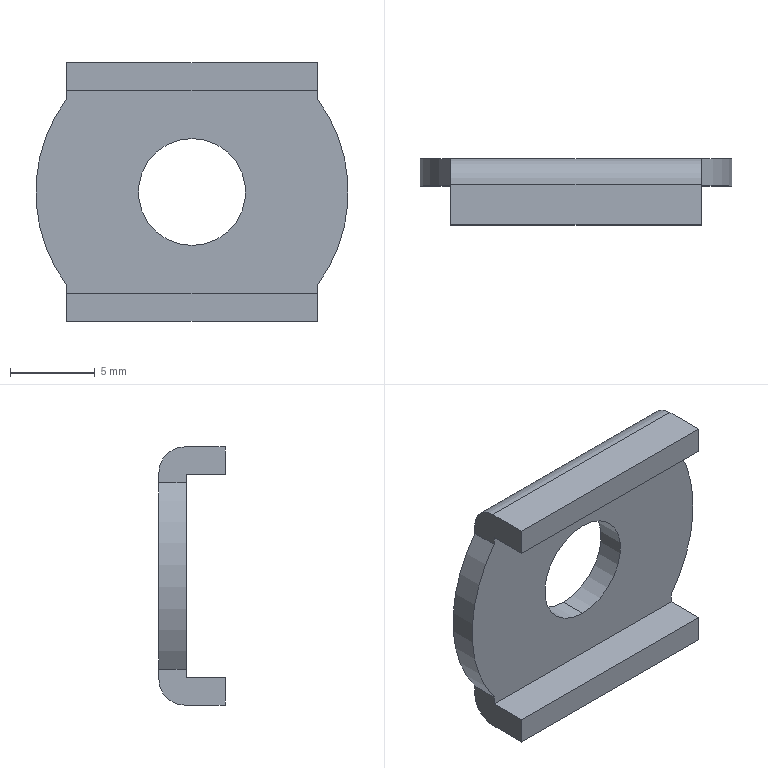Part | STEP file | 11-CLMP_MC01-S311 | 1 solid | 18 faces | box 18.4 x 3.9 x 15.2 mm | volume 446.915 mm3 | plane 12 | cylinder 6 | commonest cylinder face diameters 3 x2 6.3 x2 18.4 x2
STEP:
#1=CARTESIAN_POINT('',(0.,-1.6,-3.15));
#2=VERTEX_POINT('',#1);
#3=CARTESIAN_POINT('',(0.,-1.6,3.15));
#4=VERTEX_POINT('',#3);
#5=CARTESIAN_POINT('',(0.,-1.6,0.));
#6=DIRECTION('',(0.,1.,0.));
#7=DIRECTION('',(0.,0.,1.));
#8=AXIS2_PLACEMENT_3D('',#5,#6,#7);
#9=CIRCLE('',#8,3.15);
#10=EDGE_CURVE('',#2,#4,#9,.T.);
#11=ORIENTED_EDGE('',*,*,#10,.F.);
#12=CARTESIAN_POINT('',(0.,0.,-3.15));
#13=VERTEX_POINT('',#12);
#14=CARTESIAN_POINT('',(0.,0.,-3.15));
#15=DIRECTION('',(0.,1.,0.));
#16=VECTOR('',#15,1000.);
#17=LINE('',#14,#16);
#18=EDGE_CURVE('',#2,#13,#17,.T.);
#19=ORIENTED_EDGE('',*,*,#18,.T.);
#20=CARTESIAN_POINT('',(0.,0.,3.15));
#21=VERTEX_POINT('',#20);
#22=CARTESIAN_POINT('',(0.,0.,0.));
#23=DIRECTION('',(0.,1.,0.));
#24=DIRECTION('',(0.,0.,1.));
#25=AXIS2_PLACEMENT_3D('',#22,#23,#24);
#26=CIRCLE('',#25,3.15);
#27=EDGE_CURVE('',#13,#21,#26,.T.);
#28=ORIENTED_EDGE('',*,*,#27,.T.);
#29=CARTESIAN_POINT('',(0.,0.,3.15));
#30=DIRECTION('',(0.,1.,0.));
#31=VECTOR('',#30,1000.);
#32=LINE('',#29,#31);
#33=EDGE_CURVE('',#4,#21,#32,.T.);
#34=ORIENTED_EDGE('',*,*,#33,.F.);
#35=EDGE_LOOP('',(#11,#19,#28,#34));
#36=FACE_OUTER_BOUND('',#35,.T.);
#37=CARTESIAN_POINT('',(0.,0.,0.));
#38=DIRECTION('',(0.,1.,0.));
#39=DIRECTION('',(0.,0.,1.));
#40=AXIS2_PLACEMENT_3D('',#37,#38,#39);
#41=CYLINDRICAL_SURFACE('',#40,3.15);
#42=ADVANCED_FACE('',(#36),#41,.F.);
#43=CARTESIAN_POINT('',(-7.375,-1.6,-5.5));
#44=VERTEX_POINT('',#43);
#45=CARTESIAN_POINT('',(-7.375,0.,-5.5));
#46=VERTEX_POINT('',#45);
#47=CARTESIAN_POINT('',(-7.375,-3.9,-5.5));
#48=DIRECTION('',(0.,1.,0.));
#49=VECTOR('',#48,1000.);
#50=LINE('',#47,#49);
#51=EDGE_CURVE('',#44,#46,#50,.T.);
#52=ORIENTED_EDGE('',*,*,#51,.F.);
#53=CARTESIAN_POINT('',(-7.375,-1.6,5.5));
#54=VERTEX_POINT('',#53);
#55=CARTESIAN_POINT('',(0.,-1.6,0.));
#56=DIRECTION('',(0.,1.,0.));
#57=DIRECTION('',(0.,0.,1.));
#58=AXIS2_PLACEMENT_3D('',#55,#56,#57);
#59=CIRCLE('',#58,9.2);
#60=EDGE_CURVE('',#44,#54,#59,.T.);
#61=ORIENTED_EDGE('',*,*,#60,.T.);
#62=CARTESIAN_POINT('',(-7.375,0.,5.5));
#63=VERTEX_POINT('',#62);
#64=CARTESIAN_POINT('',(-7.375,-3.9,5.5));
#65=DIRECTION('',(0.,1.,0.));
#66=VECTOR('',#65,1000.);
#67=LINE('',#64,#66);
#68=EDGE_CURVE('',#54,#63,#67,.T.);
#69=ORIENTED_EDGE('',*,*,#68,.T.);
#70=CARTESIAN_POINT('',(0.,0.,0.));
#71=DIRECTION('',(0.,1.,0.));
#72=DIRECTION('',(0.,0.,1.));
#73=AXIS2_PLACEMENT_3D('',#70,#71,#72);
#74=CIRCLE('',#73,9.2);
#75=EDGE_CURVE('',#46,#63,#74,.T.);
#76=ORIENTED_EDGE('',*,*,#75,.F.);
#77=EDGE_LOOP('',(#52,#61,#69,#76));
#78=FACE_OUTER_BOUND('',#77,.T.);
#79=CARTESIAN_POINT('',(0.,-3.9,0.));
#80=DIRECTION('',(0.,1.,0.));
#81=DIRECTION('',(0.,0.,1.));
#82=AXIS2_PLACEMENT_3D('',#79,#80,#81);
#83=CYLINDRICAL_SURFACE('',#82,9.2);
#84=ADVANCED_FACE('',(#78),#83,.T.);
#85=CARTESIAN_POINT('',(-7.375,-3.9,-6.));
#86=VERTEX_POINT('',#85);
#87=CARTESIAN_POINT('',(-7.375,-1.6,-6.));
#88=VERTEX_POINT('',#87);
#89=CARTESIAN_POINT('',(-7.375,-3.9,-6.));
#90=DIRECTION('',(0.,1.,0.));
#91=VECTOR('',#90,1000.);
#92=LINE('',#89,#91);
#93=EDGE_CURVE('',#86,#88,#92,.T.);
#94=ORIENTED_EDGE('',*,*,#93,.T.);
#95=CARTESIAN_POINT('',(-7.375,-1.6,0.));
#96=DIRECTION('',(0.,0.,1.));
#97=VECTOR('',#96,1000.);
#98=LINE('',#95,#97);
#99=EDGE_CURVE('',#88,#44,#98,.T.);
#100=ORIENTED_EDGE('',*,*,#99,.T.);
#101=ORIENTED_EDGE('',*,*,#51,.T.);
#102=CARTESIAN_POINT('',(-7.375,0.,-6.1));
#103=VERTEX_POINT('',#102);
#104=CARTESIAN_POINT('',(-7.375,0.,-5.5));
#105=DIRECTION('',(0.,0.,1.));
#106=VECTOR('',#105,1000.);
#107=LINE('',#104,#106);
#108=EDGE_CURVE('',#103,#46,#107,.T.);
#109=ORIENTED_EDGE('',*,*,#108,.F.);
#110=CARTESIAN_POINT('',(-7.375,-1.5,-7.6));
#111=VERTEX_POINT('',#110);
#112=CARTESIAN_POINT('',(-7.375,-1.5,-6.1));
#113=DIRECTION('',(-1.,0.,0.));
#114=DIRECTION('',(0.,0.,1.));
#115=AXIS2_PLACEMENT_3D('',#112,#113,#114);
#116=CIRCLE('',#115,1.5);
#117=EDGE_CURVE('',#103,#111,#116,.T.);
#118=ORIENTED_EDGE('',*,*,#117,.T.);
#119=CARTESIAN_POINT('',(-7.375,-3.9,-7.6));
#120=VERTEX_POINT('',#119);
#121=CARTESIAN_POINT('',(-7.375,-3.9,-7.6));
#122=DIRECTION('',(0.,1.,0.));
#123=VECTOR('',#122,1000.);
#124=LINE('',#121,#123);
#125=EDGE_CURVE('',#120,#111,#124,.T.);
#126=ORIENTED_EDGE('',*,*,#125,.F.);
#127=CARTESIAN_POINT('',(-7.375,-3.9,-5.5));
#128=DIRECTION('',(0.,0.,1.));
#129=VECTOR('',#128,1000.);
#130=LINE('',#127,#129);
#131=EDGE_CURVE('',#120,#86,#130,.T.);
#132=ORIENTED_EDGE('',*,*,#131,.T.);
#133=EDGE_LOOP('',(#94,#100,#101,#109,#118,#126,#132));
#134=FACE_OUTER_BOUND('',#133,.T.);
#135=CARTESIAN_POINT('',(-7.375,-3.9,-5.5));
#136=DIRECTION('',(-1.,0.,0.));
#137=DIRECTION('',(0.,0.,1.));
#138=AXIS2_PLACEMENT_3D('',#135,#136,#137);
#139=PLANE('',#138);
#140=ADVANCED_FACE('',(#134),#139,.T.);
#141=CARTESIAN_POINT('',(7.375,-1.6,5.5));
#142=VERTEX_POINT('',#141);
#143=CARTESIAN_POINT('',(7.375,0.,5.5));
#144=VERTEX_POINT('',#143);
#145=CARTESIAN_POINT('',(7.375,-3.9,5.5));
#146=DIRECTION('',(0.,1.,0.));
#147=VECTOR('',#146,1000.);
#148=LINE('',#145,#147);
#149=EDGE_CURVE('',#142,#144,#148,.T.);
#150=ORIENTED_EDGE('',*,*,#149,.F.);
#151=CARTESIAN_POINT('',(7.375,-1.6,-5.5));
#152=VERTEX_POINT('',#151);
#153=CARTESIAN_POINT('',(0.,-1.6,0.));
#154=DIRECTION('',(0.,1.,0.));
#155=DIRECTION('',(0.,0.,1.));
#156=AXIS2_PLACEMENT_3D('',#153,#154,#155);
#157=CIRCLE('',#156,9.2);
#158=EDGE_CURVE('',#142,#152,#157,.T.);
#159=ORIENTED_EDGE('',*,*,#158,.T.);
#160=CARTESIAN_POINT('',(7.375,0.,-5.5));
#161=VERTEX_POINT('',#160);
#162=CARTESIAN_POINT('',(7.375,-3.9,-5.5));
#163=DIRECTION('',(0.,1.,0.));
#164=VECTOR('',#163,1000.);
#165=LINE('',#162,#164);
#166=EDGE_CURVE('',#152,#161,#165,.T.);
#167=ORIENTED_EDGE('',*,*,#166,.T.);
#168=CARTESIAN_POINT('',(0.,0.,0.));
#169=DIRECTION('',(0.,1.,0.));
#170=DIRECTION('',(0.,0.,1.));
#171=AXIS2_PLACEMENT_3D('',#168,#169,#170);
#172=CIRCLE('',#171,9.2);
#173=EDGE_CURVE('',#144,#161,#172,.T.);
#174=ORIENTED_EDGE('',*,*,#173,.F.);
#175=EDGE_LOOP('',(#150,#159,#167,#174));
#176=FACE_OUTER_BOUND('',#175,.T.);
#177=CARTESIAN_POINT('',(0.,-3.9,0.));
#178=DIRECTION('',(0.,1.,0.));
#179=DIRECTION('',(0.,0.,1.));
#180=AXIS2_PLACEMENT_3D('',#177,#178,#179);
#181=CYLINDRICAL_SURFACE('',#180,9.2);
#182=ADVANCED_FACE('',(#176),#181,.T.);
#183=CARTESIAN_POINT('',(7.375,-3.9,6.));
#184=VERTEX_POINT('',#183);
#185=CARTESIAN_POINT('',(7.375,-1.6,6.));
#186=VERTEX_POINT('',#185);
#187=CARTESIAN_POINT('',(7.375,-3.9,6.));
#188=DIRECTION('',(0.,1.,0.));
#189=VECTOR('',#188,1000.);
#190=LINE('',#187,#189);
#191=EDGE_CURVE('',#184,#186,#190,.T.);
#192=ORIENTED_EDGE('',*,*,#191,.T.);
#193=CARTESIAN_POINT('',(7.375,-1.6,0.));
#194=DIRECTION('',(0.,0.,-1.));
#195=VECTOR('',#194,1000.);
#196=LINE('',#193,#195);
#197=EDGE_CURVE('',#186,#142,#196,.T.);
#198=ORIENTED_EDGE('',*,*,#197,.T.);
#199=ORIENTED_EDGE('',*,*,#149,.T.);
#200=CARTESIAN_POINT('',(7.375,0.,6.1));
#201=VERTEX_POINT('',#200);
#202=CARTESIAN_POINT('',(7.375,0.,7.6));
#203=DIRECTION('',(0.,0.,-1.));
#204=VECTOR('',#203,1000.);
#205=LINE('',#202,#204);
#206=EDGE_CURVE('',#201,#144,#205,.T.);
#207=ORIENTED_EDGE('',*,*,#206,.F.);
#208=CARTESIAN_POINT('',(7.375,-1.5,7.6));
#209=VERTEX_POINT('',#208);
#210=CARTESIAN_POINT('',(7.375,-1.5,6.1));
#211=DIRECTION('',(1.,0.,0.));
#212=DIRECTION('',(0.,0.,-1.));
#213=AXIS2_PLACEMENT_3D('',#210,#211,#212);
#214=CIRCLE('',#213,1.5);
#215=EDGE_CURVE('',#201,#209,#214,.T.);
#216=ORIENTED_EDGE('',*,*,#215,.T.);
#217=CARTESIAN_POINT('',(7.375,-3.9,7.6));
#218=VERTEX_POINT('',#217);
#219=CARTESIAN_POINT('',(7.375,-3.9,7.6));
#220=DIRECTION('',(0.,1.,0.));
#221=VECTOR('',#220,1000.);
#222=LINE('',#219,#221);
#223=EDGE_CURVE('',#218,#209,#222,.T.);
#224=ORIENTED_EDGE('',*,*,#223,.F.);
#225=CARTESIAN_POINT('',(7.375,-3.9,7.6));
#226=DIRECTION('',(0.,0.,-1.));
#227=VECTOR('',#226,1000.);
#228=LINE('',#225,#227);
#229=EDGE_CURVE('',#218,#184,#228,.T.);
#230=ORIENTED_EDGE('',*,*,#229,.T.);
#231=EDGE_LOOP('',(#192,#198,#199,#207,#216,#224,#230));
#232=FACE_OUTER_BOUND('',#231,.T.);
#233=CARTESIAN_POINT('',(7.375,-3.9,7.6));
#234=DIRECTION('',(1.,0.,0.));
#235=DIRECTION('',(0.,0.,-1.));
#236=AXIS2_PLACEMENT_3D('',#233,#234,#235);
#237=PLANE('',#236);
#238=ADVANCED_FACE('',(#232),#237,.T.);
#239=CARTESIAN_POINT('',(7.375,-3.9,-6.));
#240=VERTEX_POINT('',#239);
#241=CARTESIAN_POINT('',(7.375,-3.9,-7.6));
#242=VERTEX_POINT('',#241);
#243=CARTESIAN_POINT('',(7.375,-3.9,-5.5));
#244=DIRECTION('',(0.,0.,-1.));
#245=VECTOR('',#244,1000.);
#246=LINE('',#243,#245);
#247=EDGE_CURVE('',#240,#242,#246,.T.);
#248=ORIENTED_EDGE('',*,*,#247,.F.);
#249=CARTESIAN_POINT('',(0.,-3.9,-6.));
#250=DIRECTION('',(-1.,0.,0.));
#251=VECTOR('',#250,1000.);
#252=LINE('',#249,#251);
#253=EDGE_CURVE('',#240,#86,#252,.T.);
#254=ORIENTED_EDGE('',*,*,#253,.T.);
#255=ORIENTED_EDGE('',*,*,#131,.F.);
#256=CARTESIAN_POINT('',(-7.375,-3.9,-7.6));
#257=DIRECTION('',(-1.,0.,0.));
#258=VECTOR('',#257,1000.);
#259=LINE('',#256,#258);
#260=EDGE_CURVE('',#242,#120,#259,.T.);
#261=ORIENTED_EDGE('',*,*,#260,.F.);
#262=EDGE_LOOP('',(#248,#254,#255,#261));
#263=FACE_OUTER_BOUND('',#262,.T.);
#264=CARTESIAN_POINT('',(0.,-3.9,0.));
#265=DIRECTION('',(0.,1.,0.));
#266=DIRECTION('',(0.,0.,1.));
#267=AXIS2_PLACEMENT_3D('',#264,#265,#266);
#268=PLANE('',#267);
#269=ADVANCED_FACE('',(#263),#268,.F.);
#270=ORIENTED_EDGE('',*,*,#125,.T.);
#271=CARTESIAN_POINT('',(7.375,-1.5,-7.6));
#272=VERTEX_POINT('',#271);
#273=CARTESIAN_POINT('',(-7.375,-1.5,-7.6));
#274=DIRECTION('',(1.,0.,0.));
#275=VECTOR('',#274,1000.);
#276=LINE('',#273,#275);
#277=EDGE_CURVE('',#111,#272,#276,.T.);
#278=ORIENTED_EDGE('',*,*,#277,.T.);
#279=CARTESIAN_POINT('',(7.375,-3.9,-7.6));
#280=DIRECTION('',(0.,1.,0.));
#281=VECTOR('',#280,1000.);
#282=LINE('',#279,#281);
#283=EDGE_CURVE('',#242,#272,#282,.T.);
#284=ORIENTED_EDGE('',*,*,#283,.F.);
#285=ORIENTED_EDGE('',*,*,#260,.T.);
#286=EDGE_LOOP('',(#270,#278,#284,#285));
#287=FACE_OUTER_BOUND('',#286,.T.);
#288=CARTESIAN_POINT('',(-7.375,-3.9,-7.6));
#289=DIRECTION('',(0.,0.,-1.));
#290=DIRECTION('',(-1.,0.,0.));
#291=AXIS2_PLACEMENT_3D('',#288,#289,#290);
#292=PLANE('',#291);
#293=ADVANCED_FACE('',(#287),#292,.T.);
#294=CARTESIAN_POINT('',(7.375,-1.6,-6.));
#295=VERTEX_POINT('',#294);
#296=CARTESIAN_POINT('',(7.375,-3.9,-6.));
#297=DIRECTION('',(0.,1.,0.));
#298=VECTOR('',#297,1000.);
#299=LINE('',#296,#298);
#300=EDGE_CURVE('',#240,#295,#299,.T.);
#301=ORIENTED_EDGE('',*,*,#300,.F.);
#302=ORIENTED_EDGE('',*,*,#247,.T.);
#303=ORIENTED_EDGE('',*,*,#283,.T.);
#304=CARTESIAN_POINT('',(7.375,0.,-6.1));
#305=VERTEX_POINT('',#304);
#306=CARTESIAN_POINT('',(7.375,-1.5,-6.1));
#307=DIRECTION('',(1.,0.,0.));
#308=DIRECTION('',(0.,0.,-1.));
#309=AXIS2_PLACEMENT_3D('',#306,#307,#308);
#310=CIRCLE('',#309,1.5);
#311=EDGE_CURVE('',#272,#305,#310,.T.);
#312=ORIENTED_EDGE('',*,*,#311,.T.);
#313=CARTESIAN_POINT('',(7.375,0.,-5.5));
#314=DIRECTION('',(0.,0.,-1.));
#315=VECTOR('',#314,1000.);
#316=LINE('',#313,#315);
#317=EDGE_CURVE('',#161,#305,#316,.T.);
#318=ORIENTED_EDGE('',*,*,#317,.F.);
#319=ORIENTED_EDGE('',*,*,#166,.F.);
#320=CARTESIAN_POINT('',(7.375,-1.6,0.));
#321=DIRECTION('',(0.,0.,-1.));
#322=VECTOR('',#321,1000.);
#323=LINE('',#320,#322);
#324=EDGE_CURVE('',#152,#295,#323,.T.);
#325=ORIENTED_EDGE('',*,*,#324,.T.);
#326=EDGE_LOOP('',(#301,#302,#303,#312,#318,#319,#325));
#327=FACE_OUTER_BOUND('',#326,.T.);
#328=CARTESIAN_POINT('',(7.375,-3.9,-5.5));
#329=DIRECTION('',(1.,0.,0.));
#330=DIRECTION('',(0.,0.,-1.));
#331=AXIS2_PLACEMENT_3D('',#328,#329,#330);
#332=PLANE('',#331);
#333=ADVANCED_FACE('',(#327),#332,.T.);
#334=ORIENTED_EDGE('',*,*,#223,.T.);
#335=CARTESIAN_POINT('',(-7.375,-1.5,7.6));
#336=VERTEX_POINT('',#335);
#337=CARTESIAN_POINT('',(-7.375,-1.5,7.6));
#338=DIRECTION('',(-1.,0.,0.));
#339=VECTOR('',#338,1000.);
#340=LINE('',#337,#339);
#341=EDGE_CURVE('',#209,#336,#340,.T.);
#342=ORIENTED_EDGE('',*,*,#341,.T.);
#343=CARTESIAN_POINT('',(-7.375,-3.9,7.6));
#344=VERTEX_POINT('',#343);
#345=CARTESIAN_POINT('',(-7.375,-3.9,7.6));
#346=DIRECTION('',(0.,1.,0.));
#347=VECTOR('',#346,1000.);
#348=LINE('',#345,#347);
#349=EDGE_CURVE('',#344,#336,#348,.T.);
#350=ORIENTED_EDGE('',*,*,#349,.F.);
#351=CARTESIAN_POINT('',(-7.375,-3.9,7.6));
#352=DIRECTION('',(1.,0.,0.));
#353=VECTOR('',#352,1000.);
#354=LINE('',#351,#353);
#355=EDGE_CURVE('',#344,#218,#354,.T.);
#356=ORIENTED_EDGE('',*,*,#355,.T.);
#357=EDGE_LOOP('',(#334,#342,#350,#356));
#358=FACE_OUTER_BOUND('',#357,.T.);
#359=CARTESIAN_POINT('',(-7.375,-3.9,7.6));
#360=DIRECTION('',(0.,0.,1.));
#361=DIRECTION('',(1.,0.,0.));
#362=AXIS2_PLACEMENT_3D('',#359,#360,#361);
#363=PLANE('',#362);
#364=ADVANCED_FACE('',(#358),#363,.T.);
#365=CARTESIAN_POINT('',(-7.375,-3.9,6.));
#366=VERTEX_POINT('',#365);
#367=CARTESIAN_POINT('',(-7.375,-1.6,6.));
#368=VERTEX_POINT('',#367);
#369=CARTESIAN_POINT('',(-7.375,-3.9,6.));
#370=DIRECTION('',(0.,1.,0.));
#371=VECTOR('',#370,1000.);
#372=LINE('',#369,#371);
#373=EDGE_CURVE('',#366,#368,#372,.T.);
#374=ORIENTED_EDGE('',*,*,#373,.F.);
#375=CARTESIAN_POINT('',(-7.375,-3.9,7.6));
#376=DIRECTION('',(0.,0.,1.));
#377=VECTOR('',#376,1000.);
#378=LINE('',#375,#377);
#379=EDGE_CURVE('',#366,#344,#378,.T.);
#380=ORIENTED_EDGE('',*,*,#379,.T.);
#381=ORIENTED_EDGE('',*,*,#349,.T.);
#382=CARTESIAN_POINT('',(-7.375,0.,6.1));
#383=VERTEX_POINT('',#382);
#384=CARTESIAN_POINT('',(-7.375,-1.5,6.1));
#385=DIRECTION('',(-1.,0.,0.));
#386=DIRECTION('',(0.,0.,1.));
#387=AXIS2_PLACEMENT_3D('',#384,#385,#386);
#388=CIRCLE('',#387,1.5);
#389=EDGE_CURVE('',#336,#383,#388,.T.);
#390=ORIENTED_EDGE('',*,*,#389,.T.);
#391=CARTESIAN_POINT('',(-7.375,0.,7.6));
#392=DIRECTION('',(0.,0.,1.));
#393=VECTOR('',#392,1000.);
#394=LINE('',#391,#393);
#395=EDGE_CURVE('',#63,#383,#394,.T.);
#396=ORIENTED_EDGE('',*,*,#395,.F.);
#397=ORIENTED_EDGE('',*,*,#68,.F.);
#398=CARTESIAN_POINT('',(-7.375,-1.6,0.));
#399=DIRECTION('',(0.,0.,1.));
#400=VECTOR('',#399,1000.);
#401=LINE('',#398,#400);
#402=EDGE_CURVE('',#54,#368,#401,.T.);
#403=ORIENTED_EDGE('',*,*,#402,.T.);
#404=EDGE_LOOP('',(#374,#380,#381,#390,#396,#397,#403));
#405=FACE_OUTER_BOUND('',#404,.T.);
#406=CARTESIAN_POINT('',(-7.375,-3.9,7.6));
#407=DIRECTION('',(-1.,0.,0.));
#408=DIRECTION('',(0.,0.,1.));
#409=AXIS2_PLACEMENT_3D('',#406,#407,#408);
#410=PLANE('',#409);
#411=ADVANCED_FACE('',(#405),#410,.T.);
#412=ORIENTED_EDGE('',*,*,#379,.F.);
#413=CARTESIAN_POINT('',(0.,-3.9,6.));
#414=DIRECTION('',(1.,0.,0.));
#415=VECTOR('',#414,1000.);
#416=LINE('',#413,#415);
#417=EDGE_CURVE('',#366,#184,#416,.T.);
#418=ORIENTED_EDGE('',*,*,#417,.T.);
#419=ORIENTED_EDGE('',*,*,#229,.F.);
#420=ORIENTED_EDGE('',*,*,#355,.F.);
#421=EDGE_LOOP('',(#412,#418,#419,#420));
#422=FACE_OUTER_BOUND('',#421,.T.);
#423=CARTESIAN_POINT('',(0.,-3.9,0.));
#424=DIRECTION('',(0.,1.,0.));
#425=DIRECTION('',(0.,0.,1.));
#426=AXIS2_PLACEMENT_3D('',#423,#424,#425);
#427=PLANE('',#426);
#428=ADVANCED_FACE('',(#422),#427,.F.);
#429=CARTESIAN_POINT('',(0.,0.,0.));
#430=DIRECTION('',(0.,1.,0.));
#431=DIRECTION('',(0.,0.,1.));
#432=AXIS2_PLACEMENT_3D('',#429,#430,#431);
#433=CIRCLE('',#432,3.15);
#434=EDGE_CURVE('',#21,#13,#433,.T.);
#435=ORIENTED_EDGE('',*,*,#434,.F.);
#436=ORIENTED_EDGE('',*,*,#27,.F.);
#437=EDGE_LOOP('',(#435,#436));
#438=FACE_BOUND('',#437,.T.);
#439=ORIENTED_EDGE('',*,*,#317,.T.);
#440=CARTESIAN_POINT('',(0.,0.,-6.1));
#441=DIRECTION('',(-1.,0.,0.));
#442=VECTOR('',#441,1000.);
#443=LINE('',#440,#442);
#444=EDGE_CURVE('',#305,#103,#443,.T.);
#445=ORIENTED_EDGE('',*,*,#444,.T.);
#446=ORIENTED_EDGE('',*,*,#108,.T.);
#447=ORIENTED_EDGE('',*,*,#75,.T.);
#448=ORIENTED_EDGE('',*,*,#395,.T.);
#449=CARTESIAN_POINT('',(0.,0.,6.1));
#450=DIRECTION('',(1.,0.,0.));
#451=VECTOR('',#450,1000.);
#452=LINE('',#449,#451);
#453=EDGE_CURVE('',#383,#201,#452,.T.);
#454=ORIENTED_EDGE('',*,*,#453,.T.);
#455=ORIENTED_EDGE('',*,*,#206,.T.);
#456=ORIENTED_EDGE('',*,*,#173,.T.);
#457=EDGE_LOOP('',(#439,#445,#446,#447,#448,#454,#455,#456));
#458=FACE_OUTER_BOUND('',#457,.T.);
#459=CARTESIAN_POINT('',(0.,0.,0.));
#460=DIRECTION('',(0.,1.,0.));
#461=DIRECTION('',(0.,0.,1.));
#462=AXIS2_PLACEMENT_3D('',#459,#460,#461);
#463=PLANE('',#462);
#464=ADVANCED_FACE('',(#438,#458),#463,.T.);
#465=ORIENTED_EDGE('',*,*,#311,.F.);
#466=ORIENTED_EDGE('',*,*,#277,.F.);
#467=ORIENTED_EDGE('',*,*,#117,.F.);
#468=ORIENTED_EDGE('',*,*,#444,.F.);
#469=EDGE_LOOP('',(#465,#466,#467,#468));
#470=FACE_OUTER_BOUND('',#469,.T.);
#471=CARTESIAN_POINT('',(0.,-1.5,-6.1));
#472=DIRECTION('',(-1.,0.,0.));
#473=DIRECTION('',(0.,0.,1.));
#474=AXIS2_PLACEMENT_3D('',#471,#472,#473);
#475=CYLINDRICAL_SURFACE('',#474,1.5);
#476=ADVANCED_FACE('',(#470),#475,.T.);
#477=ORIENTED_EDGE('',*,*,#389,.F.);
#478=ORIENTED_EDGE('',*,*,#341,.F.);
#479=ORIENTED_EDGE('',*,*,#215,.F.);
#480=ORIENTED_EDGE('',*,*,#453,.F.);
#481=EDGE_LOOP('',(#477,#478,#479,#480));
#482=FACE_OUTER_BOUND('',#481,.T.);
#483=CARTESIAN_POINT('',(0.,-1.5,6.1));
#484=DIRECTION('',(1.,0.,0.));
#485=DIRECTION('',(0.,0.,-1.));
#486=AXIS2_PLACEMENT_3D('',#483,#484,#485);
#487=CYLINDRICAL_SURFACE('',#486,1.5);
#488=ADVANCED_FACE('',(#482),#487,.T.);
#489=ORIENTED_EDGE('',*,*,#93,.F.);
#490=ORIENTED_EDGE('',*,*,#253,.F.);
#491=ORIENTED_EDGE('',*,*,#300,.T.);
#492=CARTESIAN_POINT('',(-7.375,-1.6,-6.));
#493=DIRECTION('',(1.,0.,0.));
#494=VECTOR('',#493,1000.);
#495=LINE('',#492,#494);
#496=EDGE_CURVE('',#88,#295,#495,.T.);
#497=ORIENTED_EDGE('',*,*,#496,.F.);
#498=EDGE_LOOP('',(#489,#490,#491,#497));
#499=FACE_OUTER_BOUND('',#498,.T.);
#500=CARTESIAN_POINT('',(-7.375,-3.9,-6.));
#501=DIRECTION('',(0.,0.,-1.));
#502=DIRECTION('',(-1.,0.,0.));
#503=AXIS2_PLACEMENT_3D('',#500,#501,#502);
#504=PLANE('',#503);
#505=ADVANCED_FACE('',(#499),#504,.F.);
#506=ORIENTED_EDGE('',*,*,#191,.F.);
#507=ORIENTED_EDGE('',*,*,#417,.F.);
#508=ORIENTED_EDGE('',*,*,#373,.T.);
#509=CARTESIAN_POINT('',(-7.375,-1.6,6.));
#510=DIRECTION('',(-1.,0.,0.));
#511=VECTOR('',#510,1000.);
#512=LINE('',#509,#511);
#513=EDGE_CURVE('',#186,#368,#512,.T.);
#514=ORIENTED_EDGE('',*,*,#513,.F.);
#515=EDGE_LOOP('',(#506,#507,#508,#514));
#516=FACE_OUTER_BOUND('',#515,.T.);
#517=CARTESIAN_POINT('',(-7.375,-3.9,6.));
#518=DIRECTION('',(0.,0.,1.));
#519=DIRECTION('',(1.,0.,0.));
#520=AXIS2_PLACEMENT_3D('',#517,#518,#519);
#521=PLANE('',#520);
#522=ADVANCED_FACE('',(#516),#521,.F.);
#523=CARTESIAN_POINT('',(0.,-1.6,0.));
#524=DIRECTION('',(0.,1.,0.));
#525=DIRECTION('',(0.,0.,1.));
#526=AXIS2_PLACEMENT_3D('',#523,#524,#525);
#527=CIRCLE('',#526,3.15);
#528=EDGE_CURVE('',#4,#2,#527,.T.);
#529=ORIENTED_EDGE('',*,*,#528,.T.);
#530=ORIENTED_EDGE('',*,*,#10,.T.);
#531=EDGE_LOOP('',(#529,#530));
#532=FACE_BOUND('',#531,.T.);
#533=ORIENTED_EDGE('',*,*,#324,.F.);
#534=ORIENTED_EDGE('',*,*,#158,.F.);
#535=ORIENTED_EDGE('',*,*,#197,.F.);
#536=ORIENTED_EDGE('',*,*,#513,.T.);
#537=ORIENTED_EDGE('',*,*,#402,.F.);
#538=ORIENTED_EDGE('',*,*,#60,.F.);
#539=ORIENTED_EDGE('',*,*,#99,.F.);
#540=ORIENTED_EDGE('',*,*,#496,.T.);
#541=EDGE_LOOP('',(#533,#534,#535,#536,#537,#538,#539,#540));
#542=FACE_OUTER_BOUND('',#541,.T.);
#543=CARTESIAN_POINT('',(0.,-1.6,0.));
#544=DIRECTION('',(0.,1.,0.));
#545=DIRECTION('',(0.,0.,1.));
#546=AXIS2_PLACEMENT_3D('',#543,#544,#545);
#547=PLANE('',#546);
#548=ADVANCED_FACE('',(#532,#542),#547,.F.);
#549=ORIENTED_EDGE('',*,*,#18,.F.);
#550=ORIENTED_EDGE('',*,*,#528,.F.);
#551=ORIENTED_EDGE('',*,*,#33,.T.);
#552=ORIENTED_EDGE('',*,*,#434,.T.);
#553=EDGE_LOOP('',(#549,#550,#551,#552));
#554=FACE_OUTER_BOUND('',#553,.T.);
#555=CARTESIAN_POINT('',(0.,0.,0.));
#556=DIRECTION('',(0.,1.,0.));
#557=DIRECTION('',(0.,0.,1.));
#558=AXIS2_PLACEMENT_3D('',#555,#556,#557);
#559=CYLINDRICAL_SURFACE('',#558,3.15);
#560=ADVANCED_FACE('',(#554),#559,.F.);
#561=CLOSED_SHELL('',(#42,#84,#140,#182,#238,#269,#293,#333,#364,#411,#428,#464,#476,#488,#505,#522,#548,#560));
#562=MANIFOLD_SOLID_BREP('',#561);
#563=CARTESIAN_POINT('',(0.,0.,0.));
#564=DIRECTION('',(0.,0.,1.));
#565=DIRECTION('',(1.,0.,0.));
#566=AXIS2_PLACEMENT_3D('',#563,#564,#565);
#567=(LENGTH_UNIT()NAMED_UNIT(*)SI_UNIT(.MILLI.,.METRE.));
#568=UNCERTAINTY_MEASURE_WITH_UNIT(LENGTH_MEASURE(0.00001),#567,'','');
#569=(NAMED_UNIT(*)PLANE_ANGLE_UNIT()SI_UNIT($,.RADIAN.));
#570=(NAMED_UNIT(*)SI_UNIT($,.STERADIAN.)SOLID_ANGLE_UNIT());
#571=(GEOMETRIC_REPRESENTATION_CONTEXT(3)GLOBAL_UNCERTAINTY_ASSIGNED_CONTEXT((#568))GLOBAL_UNIT_ASSIGNED_CONTEXT((#567,#569,#570))REPRESENTATION_CONTEXT('',''));
#572=ADVANCED_BREP_SHAPE_REPRESENTATION('',(#562,#566),#571);